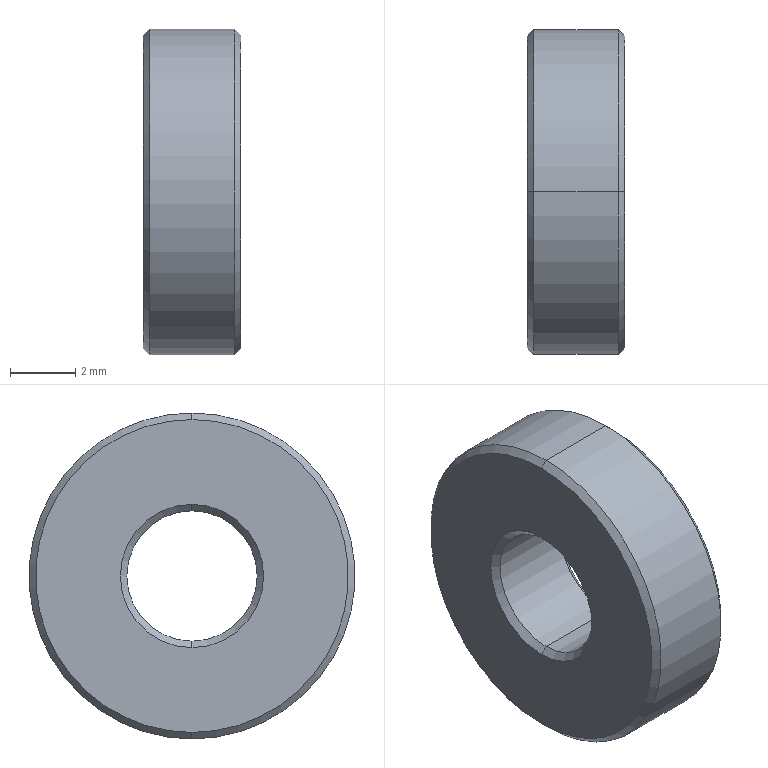Part | STEP file | WSSS10-4-3-13 | 1 solid | 14 faces | box 3 x 10 x 10 mm | volume 196.161 mm3 | cone 8 | cylinder 4 | plane 2 | commonest cylinder face diameters 4 x2 10 x2
STEP:
#1=CARTESIAN_POINT('',(3.,0.,-4.8));
#2=VERTEX_POINT('',#1);
#3=CARTESIAN_POINT('',(3.,0.,4.8));
#4=VERTEX_POINT('',#3);
#5=CARTESIAN_POINT('',(3.,0.,0.));
#6=DIRECTION('',(1.,0.,0.));
#7=DIRECTION('',(0.,0.,1.));
#8=AXIS2_PLACEMENT_3D('',#5,#6,#7);
#9=CIRCLE('',#8,4.8);
#10=EDGE_CURVE('',#2,#4,#9,.T.);
#11=ORIENTED_EDGE('',*,*,#10,.F.);
#12=CARTESIAN_POINT('',(2.8,0.,-5.));
#13=VERTEX_POINT('',#12);
#14=CARTESIAN_POINT('',(2.8,0.,-5.));
#15=DIRECTION('',(-0.7071,0.,-0.7071));
#16=VECTOR('',#15,1000.);
#17=LINE('',#14,#16);
#18=EDGE_CURVE('',#2,#13,#17,.T.);
#19=ORIENTED_EDGE('',*,*,#18,.T.);
#20=CARTESIAN_POINT('',(2.8,0.,5.));
#21=VERTEX_POINT('',#20);
#22=CARTESIAN_POINT('',(2.8,0.,0.));
#23=DIRECTION('',(-1.,0.,0.));
#24=DIRECTION('',(0.,0.,1.));
#25=AXIS2_PLACEMENT_3D('',#22,#23,#24);
#26=CIRCLE('',#25,5.);
#27=EDGE_CURVE('',#21,#13,#26,.T.);
#28=ORIENTED_EDGE('',*,*,#27,.F.);
#29=CARTESIAN_POINT('',(2.8,0.,5.));
#30=DIRECTION('',(-0.7071,0.,0.7071));
#31=VECTOR('',#30,1000.);
#32=LINE('',#29,#31);
#33=EDGE_CURVE('',#4,#21,#32,.T.);
#34=ORIENTED_EDGE('',*,*,#33,.F.);
#35=EDGE_LOOP('',(#11,#19,#28,#34));
#36=FACE_OUTER_BOUND('',#35,.T.);
#37=CARTESIAN_POINT('',(2.8,0.,0.));
#38=DIRECTION('',(-1.,0.,0.));
#39=DIRECTION('',(0.,0.,1.));
#40=AXIS2_PLACEMENT_3D('',#37,#38,#39);
#41=CONICAL_SURFACE('',#40,5.,0.7854);
#42=ADVANCED_FACE('',(#36),#41,.T.);
#43=CARTESIAN_POINT('',(2.8,0.,2.));
#44=VERTEX_POINT('',#43);
#45=CARTESIAN_POINT('',(2.8,0.,-2.));
#46=VERTEX_POINT('',#45);
#47=CARTESIAN_POINT('',(2.8,0.,0.));
#48=DIRECTION('',(1.,0.,0.));
#49=DIRECTION('',(0.,0.,1.));
#50=AXIS2_PLACEMENT_3D('',#47,#48,#49);
#51=CIRCLE('',#50,2.);
#52=EDGE_CURVE('',#44,#46,#51,.T.);
#53=ORIENTED_EDGE('',*,*,#52,.F.);
#54=CARTESIAN_POINT('',(3.,0.,2.2));
#55=VERTEX_POINT('',#54);
#56=CARTESIAN_POINT('',(3.,0.,2.2));
#57=DIRECTION('',(0.7071,0.,0.7071));
#58=VECTOR('',#57,1000.);
#59=LINE('',#56,#58);
#60=EDGE_CURVE('',#44,#55,#59,.T.);
#61=ORIENTED_EDGE('',*,*,#60,.T.);
#62=CARTESIAN_POINT('',(3.,0.,-2.2));
#63=VERTEX_POINT('',#62);
#64=CARTESIAN_POINT('',(3.,0.,0.));
#65=DIRECTION('',(-1.,0.,0.));
#66=DIRECTION('',(0.,0.,1.));
#67=AXIS2_PLACEMENT_3D('',#64,#65,#66);
#68=CIRCLE('',#67,2.2);
#69=EDGE_CURVE('',#63,#55,#68,.T.);
#70=ORIENTED_EDGE('',*,*,#69,.F.);
#71=CARTESIAN_POINT('',(3.,0.,-2.2));
#72=DIRECTION('',(0.7071,0.,-0.7071));
#73=VECTOR('',#72,1000.);
#74=LINE('',#71,#73);
#75=EDGE_CURVE('',#46,#63,#74,.T.);
#76=ORIENTED_EDGE('',*,*,#75,.F.);
#77=EDGE_LOOP('',(#53,#61,#70,#76));
#78=FACE_OUTER_BOUND('',#77,.T.);
#79=CARTESIAN_POINT('',(3.,0.,0.));
#80=DIRECTION('',(1.,0.,0.));
#81=DIRECTION('',(0.,0.,-1.));
#82=AXIS2_PLACEMENT_3D('',#79,#80,#81);
#83=CONICAL_SURFACE('',#82,2.2,0.7854);
#84=ADVANCED_FACE('',(#78),#83,.F.);
#85=CARTESIAN_POINT('',(0.,0.,4.8));
#86=VERTEX_POINT('',#85);
#87=CARTESIAN_POINT('',(0.,0.,-4.8));
#88=VERTEX_POINT('',#87);
#89=CARTESIAN_POINT('',(0.,0.,0.));
#90=DIRECTION('',(-1.,0.,0.));
#91=DIRECTION('',(0.,0.,-1.));
#92=AXIS2_PLACEMENT_3D('',#89,#90,#91);
#93=CIRCLE('',#92,4.8);
#94=EDGE_CURVE('',#86,#88,#93,.T.);
#95=ORIENTED_EDGE('',*,*,#94,.F.);
#96=CARTESIAN_POINT('',(0.2,0.,5.));
#97=VERTEX_POINT('',#96);
#98=CARTESIAN_POINT('',(0.,0.,4.8));
#99=DIRECTION('',(0.7071,0.,0.7071));
#100=VECTOR('',#99,1000.);
#101=LINE('',#98,#100);
#102=EDGE_CURVE('',#86,#97,#101,.T.);
#103=ORIENTED_EDGE('',*,*,#102,.T.);
#104=CARTESIAN_POINT('',(0.2,0.,-5.));
#105=VERTEX_POINT('',#104);
#106=CARTESIAN_POINT('',(0.2,0.,0.));
#107=DIRECTION('',(1.,0.,0.));
#108=DIRECTION('',(0.,0.,-1.));
#109=AXIS2_PLACEMENT_3D('',#106,#107,#108);
#110=CIRCLE('',#109,5.);
#111=EDGE_CURVE('',#105,#97,#110,.T.);
#112=ORIENTED_EDGE('',*,*,#111,.F.);
#113=CARTESIAN_POINT('',(0.,0.,-4.8));
#114=DIRECTION('',(0.7071,0.,-0.7071));
#115=VECTOR('',#114,1000.);
#116=LINE('',#113,#115);
#117=EDGE_CURVE('',#88,#105,#116,.T.);
#118=ORIENTED_EDGE('',*,*,#117,.F.);
#119=EDGE_LOOP('',(#95,#103,#112,#118));
#120=FACE_OUTER_BOUND('',#119,.T.);
#121=CARTESIAN_POINT('',(0.,0.,0.));
#122=DIRECTION('',(1.,0.,0.));
#123=DIRECTION('',(0.,0.,-1.));
#124=AXIS2_PLACEMENT_3D('',#121,#122,#123);
#125=CONICAL_SURFACE('',#124,4.8,0.7854);
#126=ADVANCED_FACE('',(#120),#125,.T.);
#127=CARTESIAN_POINT('',(0.2,0.,-2.));
#128=VERTEX_POINT('',#127);
#129=CARTESIAN_POINT('',(0.2,0.,2.));
#130=VERTEX_POINT('',#129);
#131=CARTESIAN_POINT('',(0.2,0.,0.));
#132=DIRECTION('',(-1.,0.,0.));
#133=DIRECTION('',(0.,0.,-1.));
#134=AXIS2_PLACEMENT_3D('',#131,#132,#133);
#135=CIRCLE('',#134,2.);
#136=EDGE_CURVE('',#128,#130,#135,.T.);
#137=ORIENTED_EDGE('',*,*,#136,.F.);
#138=CARTESIAN_POINT('',(0.,0.,-2.2));
#139=VERTEX_POINT('',#138);
#140=CARTESIAN_POINT('',(0.2,0.,-2.));
#141=DIRECTION('',(-0.7071,0.,-0.7071));
#142=VECTOR('',#141,1000.);
#143=LINE('',#140,#142);
#144=EDGE_CURVE('',#128,#139,#143,.T.);
#145=ORIENTED_EDGE('',*,*,#144,.T.);
#146=CARTESIAN_POINT('',(0.,0.,2.2));
#147=VERTEX_POINT('',#146);
#148=CARTESIAN_POINT('',(0.,0.,0.));
#149=DIRECTION('',(1.,0.,0.));
#150=DIRECTION('',(0.,0.,-1.));
#151=AXIS2_PLACEMENT_3D('',#148,#149,#150);
#152=CIRCLE('',#151,2.2);
#153=EDGE_CURVE('',#147,#139,#152,.T.);
#154=ORIENTED_EDGE('',*,*,#153,.F.);
#155=CARTESIAN_POINT('',(0.2,0.,2.));
#156=DIRECTION('',(-0.7071,0.,0.7071));
#157=VECTOR('',#156,1000.);
#158=LINE('',#155,#157);
#159=EDGE_CURVE('',#130,#147,#158,.T.);
#160=ORIENTED_EDGE('',*,*,#159,.F.);
#161=EDGE_LOOP('',(#137,#145,#154,#160));
#162=FACE_OUTER_BOUND('',#161,.T.);
#163=CARTESIAN_POINT('',(0.2,0.,0.));
#164=DIRECTION('',(-1.,0.,0.));
#165=DIRECTION('',(0.,0.,1.));
#166=AXIS2_PLACEMENT_3D('',#163,#164,#165);
#167=CONICAL_SURFACE('',#166,2.,0.7854);
#168=ADVANCED_FACE('',(#162),#167,.F.);
#169=ORIENTED_EDGE('',*,*,#52,.T.);
#170=CARTESIAN_POINT('',(0.,0.,-2.));
#171=DIRECTION('',(-1.,0.,0.));
#172=VECTOR('',#171,1000.);
#173=LINE('',#170,#172);
#174=EDGE_CURVE('',#46,#128,#173,.T.);
#175=ORIENTED_EDGE('',*,*,#174,.T.);
#176=ORIENTED_EDGE('',*,*,#136,.T.);
#177=CARTESIAN_POINT('',(0.,0.,2.));
#178=DIRECTION('',(-1.,0.,0.));
#179=VECTOR('',#178,1000.);
#180=LINE('',#177,#179);
#181=EDGE_CURVE('',#44,#130,#180,.T.);
#182=ORIENTED_EDGE('',*,*,#181,.F.);
#183=EDGE_LOOP('',(#169,#175,#176,#182));
#184=FACE_OUTER_BOUND('',#183,.T.);
#185=CARTESIAN_POINT('',(0.,0.,0.));
#186=DIRECTION('',(-1.,0.,0.));
#187=DIRECTION('',(0.,0.,1.));
#188=AXIS2_PLACEMENT_3D('',#185,#186,#187);
#189=CYLINDRICAL_SURFACE('',#188,2.);
#190=ADVANCED_FACE('',(#184),#189,.F.);
#191=ORIENTED_EDGE('',*,*,#27,.T.);
#192=CARTESIAN_POINT('',(0.,0.,-5.));
#193=DIRECTION('',(-1.,0.,0.));
#194=VECTOR('',#193,1000.);
#195=LINE('',#192,#194);
#196=EDGE_CURVE('',#13,#105,#195,.T.);
#197=ORIENTED_EDGE('',*,*,#196,.T.);
#198=ORIENTED_EDGE('',*,*,#111,.T.);
#199=CARTESIAN_POINT('',(0.,0.,5.));
#200=DIRECTION('',(-1.,0.,0.));
#201=VECTOR('',#200,1000.);
#202=LINE('',#199,#201);
#203=EDGE_CURVE('',#21,#97,#202,.T.);
#204=ORIENTED_EDGE('',*,*,#203,.F.);
#205=EDGE_LOOP('',(#191,#197,#198,#204));
#206=FACE_OUTER_BOUND('',#205,.T.);
#207=CARTESIAN_POINT('',(0.,0.,0.));
#208=DIRECTION('',(-1.,0.,0.));
#209=DIRECTION('',(0.,0.,1.));
#210=AXIS2_PLACEMENT_3D('',#207,#208,#209);
#211=CYLINDRICAL_SURFACE('',#210,5.);
#212=ADVANCED_FACE('',(#206),#211,.T.);
#213=ORIENTED_EDGE('',*,*,#153,.T.);
#214=CARTESIAN_POINT('',(0.,0.,0.));
#215=DIRECTION('',(1.,0.,0.));
#216=DIRECTION('',(0.,0.,-1.));
#217=AXIS2_PLACEMENT_3D('',#214,#215,#216);
#218=CIRCLE('',#217,2.2);
#219=EDGE_CURVE('',#139,#147,#218,.T.);
#220=ORIENTED_EDGE('',*,*,#219,.T.);
#221=EDGE_LOOP('',(#213,#220));
#222=FACE_BOUND('',#221,.T.);
#223=CARTESIAN_POINT('',(0.,0.,0.));
#224=DIRECTION('',(-1.,0.,0.));
#225=DIRECTION('',(0.,0.,-1.));
#226=AXIS2_PLACEMENT_3D('',#223,#224,#225);
#227=CIRCLE('',#226,4.8);
#228=EDGE_CURVE('',#88,#86,#227,.T.);
#229=ORIENTED_EDGE('',*,*,#228,.T.);
#230=ORIENTED_EDGE('',*,*,#94,.T.);
#231=EDGE_LOOP('',(#229,#230));
#232=FACE_OUTER_BOUND('',#231,.T.);
#233=CARTESIAN_POINT('',(0.,2.,0.));
#234=DIRECTION('',(1.,0.,0.));
#235=DIRECTION('',(0.,0.,-1.));
#236=AXIS2_PLACEMENT_3D('',#233,#234,#235);
#237=PLANE('',#236);
#238=ADVANCED_FACE('',(#222,#232),#237,.F.);
#239=ORIENTED_EDGE('',*,*,#196,.F.);
#240=CARTESIAN_POINT('',(2.8,0.,0.));
#241=DIRECTION('',(-1.,0.,0.));
#242=DIRECTION('',(0.,0.,1.));
#243=AXIS2_PLACEMENT_3D('',#240,#241,#242);
#244=CIRCLE('',#243,5.);
#245=EDGE_CURVE('',#13,#21,#244,.T.);
#246=ORIENTED_EDGE('',*,*,#245,.T.);
#247=ORIENTED_EDGE('',*,*,#203,.T.);
#248=CARTESIAN_POINT('',(0.2,0.,0.));
#249=DIRECTION('',(1.,0.,0.));
#250=DIRECTION('',(0.,0.,-1.));
#251=AXIS2_PLACEMENT_3D('',#248,#249,#250);
#252=CIRCLE('',#251,5.);
#253=EDGE_CURVE('',#97,#105,#252,.T.);
#254=ORIENTED_EDGE('',*,*,#253,.T.);
#255=EDGE_LOOP('',(#239,#246,#247,#254));
#256=FACE_OUTER_BOUND('',#255,.T.);
#257=CARTESIAN_POINT('',(0.,0.,0.));
#258=DIRECTION('',(-1.,0.,0.));
#259=DIRECTION('',(0.,0.,1.));
#260=AXIS2_PLACEMENT_3D('',#257,#258,#259);
#261=CYLINDRICAL_SURFACE('',#260,5.);
#262=ADVANCED_FACE('',(#256),#261,.T.);
#263=ORIENTED_EDGE('',*,*,#69,.T.);
#264=CARTESIAN_POINT('',(3.,0.,0.));
#265=DIRECTION('',(-1.,0.,0.));
#266=DIRECTION('',(0.,0.,1.));
#267=AXIS2_PLACEMENT_3D('',#264,#265,#266);
#268=CIRCLE('',#267,2.2);
#269=EDGE_CURVE('',#55,#63,#268,.T.);
#270=ORIENTED_EDGE('',*,*,#269,.T.);
#271=EDGE_LOOP('',(#263,#270));
#272=FACE_BOUND('',#271,.T.);
#273=CARTESIAN_POINT('',(3.,0.,0.));
#274=DIRECTION('',(1.,0.,0.));
#275=DIRECTION('',(0.,0.,1.));
#276=AXIS2_PLACEMENT_3D('',#273,#274,#275);
#277=CIRCLE('',#276,4.8);
#278=EDGE_CURVE('',#4,#2,#277,.T.);
#279=ORIENTED_EDGE('',*,*,#278,.T.);
#280=ORIENTED_EDGE('',*,*,#10,.T.);
#281=EDGE_LOOP('',(#279,#280));
#282=FACE_OUTER_BOUND('',#281,.T.);
#283=CARTESIAN_POINT('',(3.,2.,0.));
#284=DIRECTION('',(-1.,0.,0.));
#285=DIRECTION('',(0.,0.,1.));
#286=AXIS2_PLACEMENT_3D('',#283,#284,#285);
#287=PLANE('',#286);
#288=ADVANCED_FACE('',(#272,#282),#287,.F.);
#289=ORIENTED_EDGE('',*,*,#174,.F.);
#290=CARTESIAN_POINT('',(2.8,0.,0.));
#291=DIRECTION('',(1.,0.,0.));
#292=DIRECTION('',(0.,0.,1.));
#293=AXIS2_PLACEMENT_3D('',#290,#291,#292);
#294=CIRCLE('',#293,2.);
#295=EDGE_CURVE('',#46,#44,#294,.T.);
#296=ORIENTED_EDGE('',*,*,#295,.T.);
#297=ORIENTED_EDGE('',*,*,#181,.T.);
#298=CARTESIAN_POINT('',(0.2,0.,0.));
#299=DIRECTION('',(-1.,0.,0.));
#300=DIRECTION('',(0.,0.,-1.));
#301=AXIS2_PLACEMENT_3D('',#298,#299,#300);
#302=CIRCLE('',#301,2.);
#303=EDGE_CURVE('',#130,#128,#302,.T.);
#304=ORIENTED_EDGE('',*,*,#303,.T.);
#305=EDGE_LOOP('',(#289,#296,#297,#304));
#306=FACE_OUTER_BOUND('',#305,.T.);
#307=CARTESIAN_POINT('',(0.,0.,0.));
#308=DIRECTION('',(-1.,0.,0.));
#309=DIRECTION('',(0.,0.,1.));
#310=AXIS2_PLACEMENT_3D('',#307,#308,#309);
#311=CYLINDRICAL_SURFACE('',#310,2.);
#312=ADVANCED_FACE('',(#306),#311,.F.);
#313=ORIENTED_EDGE('',*,*,#144,.F.);
#314=ORIENTED_EDGE('',*,*,#303,.F.);
#315=ORIENTED_EDGE('',*,*,#159,.T.);
#316=ORIENTED_EDGE('',*,*,#219,.F.);
#317=EDGE_LOOP('',(#313,#314,#315,#316));
#318=FACE_OUTER_BOUND('',#317,.T.);
#319=CARTESIAN_POINT('',(0.2,0.,0.));
#320=DIRECTION('',(-1.,0.,0.));
#321=DIRECTION('',(0.,0.,1.));
#322=AXIS2_PLACEMENT_3D('',#319,#320,#321);
#323=CONICAL_SURFACE('',#322,2.,0.7854);
#324=ADVANCED_FACE('',(#318),#323,.F.);
#325=ORIENTED_EDGE('',*,*,#102,.F.);
#326=ORIENTED_EDGE('',*,*,#228,.F.);
#327=ORIENTED_EDGE('',*,*,#117,.T.);
#328=ORIENTED_EDGE('',*,*,#253,.F.);
#329=EDGE_LOOP('',(#325,#326,#327,#328));
#330=FACE_OUTER_BOUND('',#329,.T.);
#331=CARTESIAN_POINT('',(0.,0.,0.));
#332=DIRECTION('',(1.,0.,0.));
#333=DIRECTION('',(0.,0.,-1.));
#334=AXIS2_PLACEMENT_3D('',#331,#332,#333);
#335=CONICAL_SURFACE('',#334,4.8,0.7854);
#336=ADVANCED_FACE('',(#330),#335,.T.);
#337=ORIENTED_EDGE('',*,*,#60,.F.);
#338=ORIENTED_EDGE('',*,*,#295,.F.);
#339=ORIENTED_EDGE('',*,*,#75,.T.);
#340=ORIENTED_EDGE('',*,*,#269,.F.);
#341=EDGE_LOOP('',(#337,#338,#339,#340));
#342=FACE_OUTER_BOUND('',#341,.T.);
#343=CARTESIAN_POINT('',(3.,0.,0.));
#344=DIRECTION('',(1.,0.,0.));
#345=DIRECTION('',(0.,0.,-1.));
#346=AXIS2_PLACEMENT_3D('',#343,#344,#345);
#347=CONICAL_SURFACE('',#346,2.2,0.7854);
#348=ADVANCED_FACE('',(#342),#347,.F.);
#349=ORIENTED_EDGE('',*,*,#18,.F.);
#350=ORIENTED_EDGE('',*,*,#278,.F.);
#351=ORIENTED_EDGE('',*,*,#33,.T.);
#352=ORIENTED_EDGE('',*,*,#245,.F.);
#353=EDGE_LOOP('',(#349,#350,#351,#352));
#354=FACE_OUTER_BOUND('',#353,.T.);
#355=CARTESIAN_POINT('',(2.8,0.,0.));
#356=DIRECTION('',(-1.,0.,0.));
#357=DIRECTION('',(0.,0.,1.));
#358=AXIS2_PLACEMENT_3D('',#355,#356,#357);
#359=CONICAL_SURFACE('',#358,5.,0.7854);
#360=ADVANCED_FACE('',(#354),#359,.T.);
#361=CLOSED_SHELL('',(#42,#84,#126,#168,#190,#212,#238,#262,#288,#312,#324,#336,#348,#360));
#362=MANIFOLD_SOLID_BREP('',#361);
#363=CARTESIAN_POINT('',(0.,0.,0.));
#364=DIRECTION('',(0.,0.,1.));
#365=DIRECTION('',(1.,0.,0.));
#366=AXIS2_PLACEMENT_3D('',#363,#364,#365);
#367=(LENGTH_UNIT()NAMED_UNIT(*)SI_UNIT(.MILLI.,.METRE.));
#368=UNCERTAINTY_MEASURE_WITH_UNIT(LENGTH_MEASURE(0.00001),#367,'','');
#369=(NAMED_UNIT(*)PLANE_ANGLE_UNIT()SI_UNIT($,.RADIAN.));
#370=(NAMED_UNIT(*)SI_UNIT($,.STERADIAN.)SOLID_ANGLE_UNIT());
#371=(GEOMETRIC_REPRESENTATION_CONTEXT(3)GLOBAL_UNCERTAINTY_ASSIGNED_CONTEXT((#368))GLOBAL_UNIT_ASSIGNED_CONTEXT((#367,#369,#370))REPRESENTATION_CONTEXT('',''));
#372=ADVANCED_BREP_SHAPE_REPRESENTATION('',(#362,#366),#371);